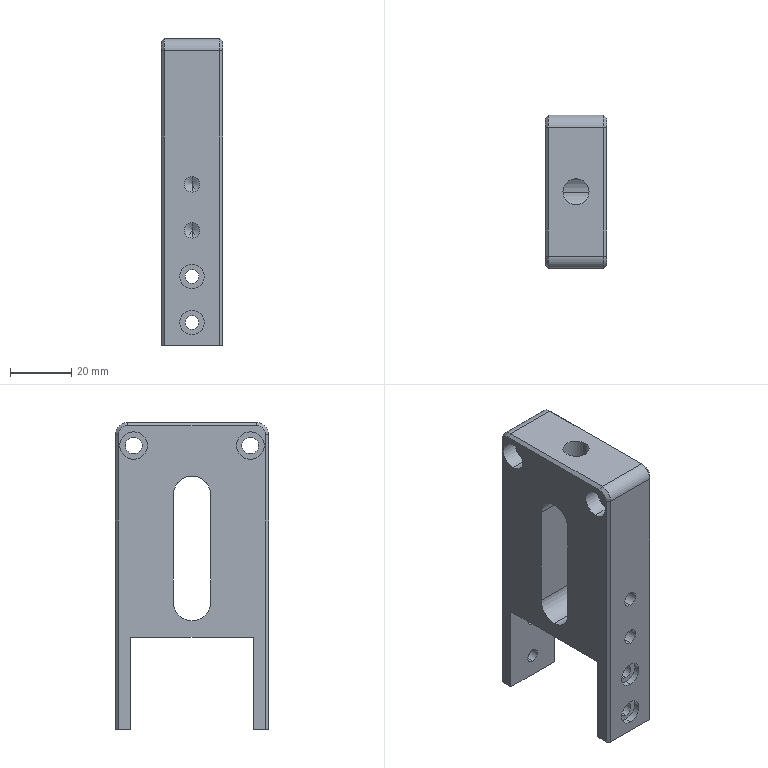Part | STEP file | 1 solid | 81 faces | box 20 x 50 x 100 mm | volume 60104 mm3 | cylinder 42 | plane 27 | cone 12 | commonest cylinder face diameters 8 x10 4.5 x8 5 x8 5.5 x4 9 x4 12.2 x3